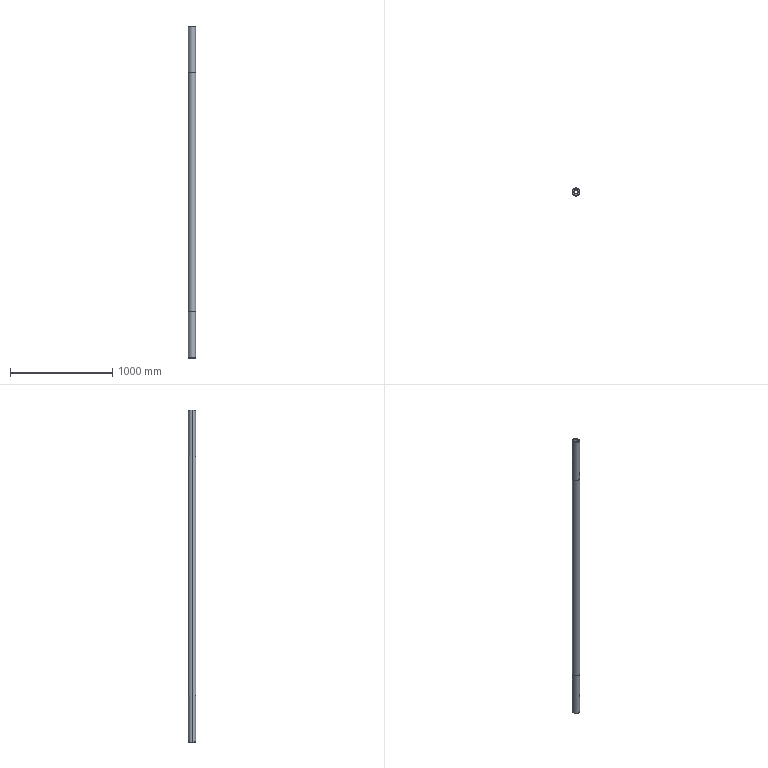Part | SolidWorks | features ICE 4, Chamfer 1, Extrusion 1, MirrorPattern 1 | 1 solid | 31 faces | box 76 x 76 x 3254 mm | volume 9186172 mm3 | cylinder 11 | cone 10 | plane 10 | commonest cylinder face diameters 70 x4 12 x3 44 x2 76 x2
STEP:
#1=CARTESIAN_POINT('',(-34.,0.,0.));
#2=VERTEX_POINT('',#1);
#3=CARTESIAN_POINT('',(-6.,33.466,0.));
#4=VERTEX_POINT('',#3);
#5=CARTESIAN_POINT('',(0.,0.,0.));
#6=DIRECTION('',(0.,0.,-1.));
#7=DIRECTION('',(1.,0.,0.));
#8=AXIS2_PLACEMENT_3D('',#5,#6,#7);
#9=CIRCLE('',#8,34.);
#10=EDGE_CURVE('',#2,#4,#9,.T.);
#11=ORIENTED_EDGE('',*,*,#10,.F.);
#12=CARTESIAN_POINT('',(-35.,0.,1.));
#13=VERTEX_POINT('',#12);
#14=CARTESIAN_POINT('',(-34.,0.,0.));
#15=DIRECTION('',(-0.7071,0.,0.7071));
#16=VECTOR('',#15,1000.);
#17=LINE('',#14,#16);
#18=EDGE_CURVE('',#2,#13,#17,.T.);
#19=ORIENTED_EDGE('',*,*,#18,.T.);
#20=CARTESIAN_POINT('',(-6.,34.482,1.));
#21=VERTEX_POINT('',#20);
#22=CARTESIAN_POINT('',(0.,0.,1.));
#23=DIRECTION('',(0.,0.,1.));
#24=DIRECTION('',(1.,0.,0.));
#25=AXIS2_PLACEMENT_3D('',#22,#23,#24);
#26=CIRCLE('',#25,35.);
#27=EDGE_CURVE('',#21,#13,#26,.T.);
#28=ORIENTED_EDGE('',*,*,#27,.F.);
#29=CARTESIAN_POINT('',(-6.,33.466,0.));
#30=CARTESIAN_POINT('',(-6.,33.805,0.3333));
#31=CARTESIAN_POINT('',(-6.,34.143,0.6666));
#32=CARTESIAN_POINT('',(-6.,34.482,1.));
#33=B_SPLINE_CURVE_WITH_KNOTS('',3,(#29,#30,#31,#32),.UNSPECIFIED.,.F.,.F.,(4,4),(0.,0.001425),.UNSPECIFIED.);
#34=EDGE_CURVE('',#4,#21,#33,.T.);
#35=ORIENTED_EDGE('',*,*,#34,.F.);
#36=EDGE_LOOP('',(#11,#19,#28,#35));
#37=FACE_OUTER_BOUND('',#36,.T.);
#38=CARTESIAN_POINT('',(0.,0.,0.));
#39=DIRECTION('',(0.,0.,1.));
#40=DIRECTION('',(1.,0.,0.));
#41=AXIS2_PLACEMENT_3D('',#38,#39,#40);
#42=CONICAL_SURFACE('',#41,34.,0.7854);
#43=ADVANCED_FACE('',(#37),#42,.T.);
#44=ORIENTED_EDGE('',*,*,#18,.F.);
#45=CARTESIAN_POINT('',(34.,0.,0.));
#46=VERTEX_POINT('',#45);
#47=CARTESIAN_POINT('',(0.,0.,0.));
#48=DIRECTION('',(0.,0.,-1.));
#49=DIRECTION('',(1.,0.,0.));
#50=AXIS2_PLACEMENT_3D('',#47,#48,#49);
#51=CIRCLE('',#50,34.);
#52=EDGE_CURVE('',#46,#2,#51,.T.);
#53=ORIENTED_EDGE('',*,*,#52,.F.);
#54=CARTESIAN_POINT('',(35.,0.,1.));
#55=VERTEX_POINT('',#54);
#56=CARTESIAN_POINT('',(34.,0.,0.));
#57=DIRECTION('',(0.7071,0.,0.7071));
#58=VECTOR('',#57,1000.);
#59=LINE('',#56,#58);
#60=EDGE_CURVE('',#46,#55,#59,.T.);
#61=ORIENTED_EDGE('',*,*,#60,.T.);
#62=CARTESIAN_POINT('',(0.,0.,1.));
#63=DIRECTION('',(0.,0.,1.));
#64=DIRECTION('',(1.,0.,0.));
#65=AXIS2_PLACEMENT_3D('',#62,#63,#64);
#66=CIRCLE('',#65,35.);
#67=EDGE_CURVE('',#13,#55,#66,.T.);
#68=ORIENTED_EDGE('',*,*,#67,.F.);
#69=EDGE_LOOP('',(#44,#53,#61,#68));
#70=FACE_OUTER_BOUND('',#69,.T.);
#71=CARTESIAN_POINT('',(0.,0.,0.));
#72=DIRECTION('',(0.,0.,1.));
#73=DIRECTION('',(1.,0.,0.));
#74=AXIS2_PLACEMENT_3D('',#71,#72,#73);
#75=CONICAL_SURFACE('',#74,34.,0.7854);
#76=ADVANCED_FACE('',(#70),#75,.T.);
#77=CARTESIAN_POINT('',(-37.,0.,453.5));
#78=VERTEX_POINT('',#77);
#79=CARTESIAN_POINT('',(37.,0.,453.5));
#80=VERTEX_POINT('',#79);
#81=CARTESIAN_POINT('',(0.,0.,453.5));
#82=DIRECTION('',(0.,0.,-1.));
#83=DIRECTION('',(-1.,0.,0.));
#84=AXIS2_PLACEMENT_3D('',#81,#82,#83);
#85=CIRCLE('',#84,37.);
#86=EDGE_CURVE('',#78,#80,#85,.T.);
#87=ORIENTED_EDGE('',*,*,#86,.F.);
#88=CARTESIAN_POINT('',(-38.,0.,454.5));
#89=VERTEX_POINT('',#88);
#90=CARTESIAN_POINT('',(-37.,0.,453.5));
#91=DIRECTION('',(-0.7071,0.,0.7071));
#92=VECTOR('',#91,1000.);
#93=LINE('',#90,#92);
#94=EDGE_CURVE('',#78,#89,#93,.T.);
#95=ORIENTED_EDGE('',*,*,#94,.T.);
#96=CARTESIAN_POINT('',(38.,0.,454.5));
#97=VERTEX_POINT('',#96);
#98=CARTESIAN_POINT('',(0.,0.,454.5));
#99=DIRECTION('',(0.,0.,1.));
#100=DIRECTION('',(-1.,0.,0.));
#101=AXIS2_PLACEMENT_3D('',#98,#99,#100);
#102=CIRCLE('',#101,38.);
#103=EDGE_CURVE('',#97,#89,#102,.T.);
#104=ORIENTED_EDGE('',*,*,#103,.F.);
#105=CARTESIAN_POINT('',(37.,0.,453.5));
#106=DIRECTION('',(0.7071,0.,0.7071));
#107=VECTOR('',#106,1000.);
#108=LINE('',#105,#107);
#109=EDGE_CURVE('',#80,#97,#108,.T.);
#110=ORIENTED_EDGE('',*,*,#109,.F.);
#111=EDGE_LOOP('',(#87,#95,#104,#110));
#112=FACE_OUTER_BOUND('',#111,.T.);
#113=CARTESIAN_POINT('',(0.,0.,453.5));
#114=DIRECTION('',(0.,0.,1.));
#115=DIRECTION('',(1.,0.,0.));
#116=AXIS2_PLACEMENT_3D('',#113,#114,#115);
#117=CONICAL_SURFACE('',#116,37.,0.7854);
#118=ADVANCED_FACE('',(#112),#117,.T.);
#119=CARTESIAN_POINT('',(37.,0.,2800.5));
#120=VERTEX_POINT('',#119);
#121=CARTESIAN_POINT('',(-37.,0.,2800.5));
#122=VERTEX_POINT('',#121);
#123=CARTESIAN_POINT('',(0.,0.,2800.5));
#124=DIRECTION('',(0.,0.,1.));
#125=DIRECTION('',(1.,0.,0.));
#126=AXIS2_PLACEMENT_3D('',#123,#124,#125);
#127=CIRCLE('',#126,37.);
#128=EDGE_CURVE('',#120,#122,#127,.T.);
#129=ORIENTED_EDGE('',*,*,#128,.F.);
#130=CARTESIAN_POINT('',(38.,0.,2799.5));
#131=VERTEX_POINT('',#130);
#132=CARTESIAN_POINT('',(37.,0.,2800.5));
#133=DIRECTION('',(0.7071,0.,-0.7071));
#134=VECTOR('',#133,1000.);
#135=LINE('',#132,#134);
#136=EDGE_CURVE('',#120,#131,#135,.T.);
#137=ORIENTED_EDGE('',*,*,#136,.T.);
#138=CARTESIAN_POINT('',(-38.,0.,2799.5));
#139=VERTEX_POINT('',#138);
#140=CARTESIAN_POINT('',(0.,0.,2799.5));
#141=DIRECTION('',(0.,0.,-1.));
#142=DIRECTION('',(1.,0.,0.));
#143=AXIS2_PLACEMENT_3D('',#140,#141,#142);
#144=CIRCLE('',#143,38.);
#145=EDGE_CURVE('',#139,#131,#144,.T.);
#146=ORIENTED_EDGE('',*,*,#145,.F.);
#147=CARTESIAN_POINT('',(-37.,0.,2800.5));
#148=DIRECTION('',(-0.7071,0.,-0.7071));
#149=VECTOR('',#148,1000.);
#150=LINE('',#147,#149);
#151=EDGE_CURVE('',#122,#139,#150,.T.);
#152=ORIENTED_EDGE('',*,*,#151,.F.);
#153=EDGE_LOOP('',(#129,#137,#146,#152));
#154=FACE_OUTER_BOUND('',#153,.T.);
#155=CARTESIAN_POINT('',(0.,0.,2800.5));
#156=DIRECTION('',(0.,0.,-1.));
#157=DIRECTION('',(-1.,0.,0.));
#158=AXIS2_PLACEMENT_3D('',#155,#156,#157);
#159=CONICAL_SURFACE('',#158,37.,0.7854);
#160=ADVANCED_FACE('',(#154),#159,.T.);
#161=CARTESIAN_POINT('',(34.,0.,3254.));
#162=VERTEX_POINT('',#161);
#163=CARTESIAN_POINT('',(6.,33.466,3254.));
#164=VERTEX_POINT('',#163);
#165=CARTESIAN_POINT('',(0.,0.,3254.));
#166=DIRECTION('',(0.,0.,1.));
#167=DIRECTION('',(1.,0.,0.));
#168=AXIS2_PLACEMENT_3D('',#165,#166,#167);
#169=CIRCLE('',#168,34.);
#170=EDGE_CURVE('',#162,#164,#169,.T.);
#171=ORIENTED_EDGE('',*,*,#170,.F.);
#172=CARTESIAN_POINT('',(35.,0.,3253.));
#173=VERTEX_POINT('',#172);
#174=CARTESIAN_POINT('',(34.,0.,3254.));
#175=DIRECTION('',(0.7071,0.,-0.7071));
#176=VECTOR('',#175,1000.);
#177=LINE('',#174,#176);
#178=EDGE_CURVE('',#162,#173,#177,.T.);
#179=ORIENTED_EDGE('',*,*,#178,.T.);
#180=CARTESIAN_POINT('',(6.,34.482,3253.));
#181=VERTEX_POINT('',#180);
#182=CARTESIAN_POINT('',(0.,0.,3253.));
#183=DIRECTION('',(0.,0.,-1.));
#184=DIRECTION('',(1.,0.,0.));
#185=AXIS2_PLACEMENT_3D('',#182,#183,#184);
#186=CIRCLE('',#185,35.);
#187=EDGE_CURVE('',#181,#173,#186,.T.);
#188=ORIENTED_EDGE('',*,*,#187,.F.);
#189=CARTESIAN_POINT('',(6.,33.466,3254.));
#190=CARTESIAN_POINT('',(6.,33.805,3253.667));
#191=CARTESIAN_POINT('',(6.,34.143,3253.333));
#192=CARTESIAN_POINT('',(6.,34.482,3253.));
#193=B_SPLINE_CURVE_WITH_KNOTS('',3,(#189,#190,#191,#192),.UNSPECIFIED.,.F.,.F.,(4,4),(0.,0.001425),.UNSPECIFIED.);
#194=EDGE_CURVE('',#164,#181,#193,.T.);
#195=ORIENTED_EDGE('',*,*,#194,.F.);
#196=EDGE_LOOP('',(#171,#179,#188,#195));
#197=FACE_OUTER_BOUND('',#196,.T.);
#198=CARTESIAN_POINT('',(0.,0.,3254.));
#199=DIRECTION('',(0.,0.,-1.));
#200=DIRECTION('',(-1.,0.,0.));
#201=AXIS2_PLACEMENT_3D('',#198,#199,#200);
#202=CONICAL_SURFACE('',#201,34.,0.7854);
#203=ADVANCED_FACE('',(#197),#202,.T.);
#204=ORIENTED_EDGE('',*,*,#178,.F.);
#205=CARTESIAN_POINT('',(-34.,0.,3254.));
#206=VERTEX_POINT('',#205);
#207=CARTESIAN_POINT('',(0.,0.,3254.));
#208=DIRECTION('',(0.,0.,1.));
#209=DIRECTION('',(1.,0.,0.));
#210=AXIS2_PLACEMENT_3D('',#207,#208,#209);
#211=CIRCLE('',#210,34.);
#212=EDGE_CURVE('',#206,#162,#211,.T.);
#213=ORIENTED_EDGE('',*,*,#212,.F.);
#214=CARTESIAN_POINT('',(-35.,0.,3253.));
#215=VERTEX_POINT('',#214);
#216=CARTESIAN_POINT('',(-34.,0.,3254.));
#217=DIRECTION('',(-0.7071,0.,-0.7071));
#218=VECTOR('',#217,1000.);
#219=LINE('',#216,#218);
#220=EDGE_CURVE('',#206,#215,#219,.T.);
#221=ORIENTED_EDGE('',*,*,#220,.T.);
#222=CARTESIAN_POINT('',(0.,0.,3253.));
#223=DIRECTION('',(0.,0.,-1.));
#224=DIRECTION('',(1.,0.,0.));
#225=AXIS2_PLACEMENT_3D('',#222,#223,#224);
#226=CIRCLE('',#225,35.);
#227=EDGE_CURVE('',#173,#215,#226,.T.);
#228=ORIENTED_EDGE('',*,*,#227,.F.);
#229=EDGE_LOOP('',(#204,#213,#221,#228));
#230=FACE_OUTER_BOUND('',#229,.T.);
#231=CARTESIAN_POINT('',(0.,0.,3254.));
#232=DIRECTION('',(0.,0.,-1.));
#233=DIRECTION('',(-1.,0.,0.));
#234=AXIS2_PLACEMENT_3D('',#231,#232,#233);
#235=CONICAL_SURFACE('',#234,34.,0.7854);
#236=ADVANCED_FACE('',(#230),#235,.T.);
#237=CARTESIAN_POINT('',(0.,31.,36.));
#238=VERTEX_POINT('',#237);
#239=CARTESIAN_POINT('',(6.,31.,30.));
#240=VERTEX_POINT('',#239);
#241=CARTESIAN_POINT('',(0.,31.,30.));
#242=DIRECTION('',(0.,1.,0.));
#243=DIRECTION('',(0.,0.,1.));
#244=AXIS2_PLACEMENT_3D('',#241,#242,#243);
#245=CIRCLE('',#244,6.);
#246=EDGE_CURVE('',#238,#240,#245,.T.);
#247=ORIENTED_EDGE('',*,*,#246,.F.);
#248=CARTESIAN_POINT('',(0.,35.,36.));
#249=VERTEX_POINT('',#248);
#250=CARTESIAN_POINT('',(0.,31.,36.));
#251=DIRECTION('',(0.,1.,0.));
#252=VECTOR('',#251,1000.);
#253=LINE('',#250,#252);
#254=EDGE_CURVE('',#238,#249,#253,.T.);
#255=ORIENTED_EDGE('',*,*,#254,.T.);
#256=CARTESIAN_POINT('',(6.,34.482,30.));
#257=VERTEX_POINT('',#256);
#258=CARTESIAN_POINT('',(0.,35.,36.));
#259=CARTESIAN_POINT('',(0.3919,35.,36.));
#260=CARTESIAN_POINT('',(0.79,34.993,35.961));
#261=CARTESIAN_POINT('',(1.559,34.967,35.807));
#262=CARTESIAN_POINT('',(1.934,34.948,35.694));
#263=CARTESIAN_POINT('',(2.479,34.913,35.468));
#264=CARTESIAN_POINT('',(2.658,34.899,35.383));
#265=CARTESIAN_POINT('',(3.005,34.871,35.197));
#266=CARTESIAN_POINT('',(3.173,34.856,35.096));
#267=CARTESIAN_POINT('',(3.659,34.81,34.771));
#268=CARTESIAN_POINT('',(3.963,34.776,34.522));
#269=CARTESIAN_POINT('',(4.521,34.708,33.964));
#270=CARTESIAN_POINT('',(4.769,34.674,33.662));
#271=CARTESIAN_POINT('',(5.094,34.627,33.176));
#272=CARTESIAN_POINT('',(5.195,34.612,33.008));
#273=CARTESIAN_POINT('',(5.381,34.584,32.661));
#274=CARTESIAN_POINT('',(5.466,34.571,32.482));
#275=CARTESIAN_POINT('',(5.692,34.534,31.938));
#276=CARTESIAN_POINT('',(5.806,34.515,31.564));
#277=CARTESIAN_POINT('',(5.96,34.489,30.794));
#278=CARTESIAN_POINT('',(6.,34.482,30.397));
#279=CARTESIAN_POINT('',(6.,34.482,30.));
#280=B_SPLINE_CURVE_WITH_KNOTS('',3,(#258,#259,#260,#261,#262,#263,#264,#265,#266,#267,#268,#269,#270,#271,#272,#273,#274,#275,#276,#277,#278,#279),.UNSPECIFIED.,.F.,.F.,(4,2,2,2,2,2,2,2,2,2,4),(0.009399,0.01057,0.01175,0.01233,0.01292,0.01409,0.01527,0.01585,0.01644,0.01761,0.01879),.UNSPECIFIED.);
#281=EDGE_CURVE('',#249,#257,#280,.T.);
#282=ORIENTED_EDGE('',*,*,#281,.T.);
#283=CARTESIAN_POINT('',(6.,31.,30.));
#284=DIRECTION('',(0.,1.,0.));
#285=VECTOR('',#284,1000.);
#286=LINE('',#283,#285);
#287=EDGE_CURVE('',#240,#257,#286,.T.);
#288=ORIENTED_EDGE('',*,*,#287,.F.);
#289=EDGE_LOOP('',(#247,#255,#282,#288));
#290=FACE_OUTER_BOUND('',#289,.T.);
#291=CARTESIAN_POINT('',(0.,31.,30.));
#292=DIRECTION('',(0.,1.,0.));
#293=DIRECTION('',(0.,0.,1.));
#294=AXIS2_PLACEMENT_3D('',#291,#292,#293);
#295=CYLINDRICAL_SURFACE('',#294,6.);
#296=ADVANCED_FACE('',(#290),#295,.F.);
#297=CARTESIAN_POINT('',(22.,0.,3254.));
#298=VERTEX_POINT('',#297);
#299=CARTESIAN_POINT('',(-22.,0.,3254.));
#300=VERTEX_POINT('',#299);
#301=CARTESIAN_POINT('',(0.,0.,3254.));
#302=DIRECTION('',(0.,0.,-1.));
#303=DIRECTION('',(-1.,0.,0.));
#304=AXIS2_PLACEMENT_3D('',#301,#302,#303);
#305=CIRCLE('',#304,22.);
#306=EDGE_CURVE('',#298,#300,#305,.T.);
#307=ORIENTED_EDGE('',*,*,#306,.F.);
#308=CARTESIAN_POINT('',(22.,0.,0.));
#309=VERTEX_POINT('',#308);
#310=CARTESIAN_POINT('',(22.,0.,3254.));
#311=DIRECTION('',(0.,0.,-1.));
#312=VECTOR('',#311,1000.);
#313=LINE('',#310,#312);
#314=EDGE_CURVE('',#298,#309,#313,.T.);
#315=ORIENTED_EDGE('',*,*,#314,.T.);
#316=CARTESIAN_POINT('',(-22.,0.,0.));
#317=VERTEX_POINT('',#316);
#318=CARTESIAN_POINT('',(0.,0.,0.));
#319=DIRECTION('',(0.,0.,-1.));
#320=DIRECTION('',(-1.,0.,0.));
#321=AXIS2_PLACEMENT_3D('',#318,#319,#320);
#322=CIRCLE('',#321,22.);
#323=EDGE_CURVE('',#309,#317,#322,.T.);
#324=ORIENTED_EDGE('',*,*,#323,.T.);
#325=CARTESIAN_POINT('',(-22.,0.,3254.));
#326=DIRECTION('',(0.,0.,-1.));
#327=VECTOR('',#326,1000.);
#328=LINE('',#325,#327);
#329=EDGE_CURVE('',#300,#317,#328,.T.);
#330=ORIENTED_EDGE('',*,*,#329,.F.);
#331=EDGE_LOOP('',(#307,#315,#324,#330));
#332=FACE_OUTER_BOUND('',#331,.T.);
#333=CARTESIAN_POINT('',(0.,0.,3254.));
#334=DIRECTION('',(0.,0.,-1.));
#335=DIRECTION('',(-1.,0.,0.));
#336=AXIS2_PLACEMENT_3D('',#333,#334,#335);
#337=CYLINDRICAL_SURFACE('',#336,22.);
#338=ADVANCED_FACE('',(#332),#337,.F.);
#339=CARTESIAN_POINT('',(-35.,0.,453.5));
#340=VERTEX_POINT('',#339);
#341=CARTESIAN_POINT('',(35.,0.,453.5));
#342=VERTEX_POINT('',#341);
#343=CARTESIAN_POINT('',(0.,0.,453.5));
#344=DIRECTION('',(0.,0.,-1.));
#345=DIRECTION('',(-1.,0.,0.));
#346=AXIS2_PLACEMENT_3D('',#343,#344,#345);
#347=CIRCLE('',#346,35.);
#348=EDGE_CURVE('',#340,#342,#347,.T.);
#349=ORIENTED_EDGE('',*,*,#348,.T.);
#350=CARTESIAN_POINT('',(35.,0.,453.5));
#351=DIRECTION('',(0.,0.,-1.));
#352=VECTOR('',#351,1000.);
#353=LINE('',#350,#352);
#354=EDGE_CURVE('',#342,#55,#353,.T.);
#355=ORIENTED_EDGE('',*,*,#354,.T.);
#356=CARTESIAN_POINT('',(6.,34.482,1.));
#357=VERTEX_POINT('',#356);
#358=CARTESIAN_POINT('',(0.,0.,1.));
#359=DIRECTION('',(0.,0.,1.));
#360=DIRECTION('',(1.,0.,0.));
#361=AXIS2_PLACEMENT_3D('',#358,#359,#360);
#362=CIRCLE('',#361,35.);
#363=EDGE_CURVE('',#55,#357,#362,.T.);
#364=ORIENTED_EDGE('',*,*,#363,.T.);
#365=CARTESIAN_POINT('',(6.,34.482,453.5));
#366=DIRECTION('',(0.,0.,-1.));
#367=VECTOR('',#366,1000.);
#368=LINE('',#365,#367);
#369=EDGE_CURVE('',#257,#357,#368,.T.);
#370=ORIENTED_EDGE('',*,*,#369,.F.);
#371=ORIENTED_EDGE('',*,*,#281,.F.);
#372=CARTESIAN_POINT('',(-6.,34.482,30.));
#373=VERTEX_POINT('',#372);
#374=CARTESIAN_POINT('',(-6.,34.482,30.));
#375=CARTESIAN_POINT('',(-6.,34.482,30.397));
#376=CARTESIAN_POINT('',(-5.961,34.489,30.788));
#377=CARTESIAN_POINT('',(-5.846,34.508,31.364));
#378=CARTESIAN_POINT('',(-5.799,34.516,31.554));
#379=CARTESIAN_POINT('',(-5.684,34.535,31.932));
#380=CARTESIAN_POINT('',(-5.617,34.546,32.119));
#381=CARTESIAN_POINT('',(-5.391,34.583,32.664));
#382=CARTESIAN_POINT('',(-5.206,34.611,33.008));
#383=CARTESIAN_POINT('',(-4.77,34.674,33.66));
#384=CARTESIAN_POINT('',(-4.517,34.708,33.968));
#385=CARTESIAN_POINT('',(-3.965,34.776,34.521));
#386=CARTESIAN_POINT('',(-3.663,34.809,34.769));
#387=CARTESIAN_POINT('',(-3.007,34.872,35.207));
#388=CARTESIAN_POINT('',(-2.659,34.901,35.393));
#389=CARTESIAN_POINT('',(-2.117,34.936,35.618));
#390=CARTESIAN_POINT('',(-1.933,34.947,35.684));
#391=CARTESIAN_POINT('',(-1.557,34.966,35.798));
#392=CARTESIAN_POINT('',(-1.364,34.974,35.846));
#393=CARTESIAN_POINT('',(-0.7822,34.993,35.962));
#394=CARTESIAN_POINT('',(-0.3923,35.,36.));
#395=CARTESIAN_POINT('',(0.,35.,36.));
#396=B_SPLINE_CURVE_WITH_KNOTS('',3,(#374,#375,#376,#377,#378,#379,#380,#381,#382,#383,#384,#385,#386,#387,#388,#389,#390,#391,#392,#393,#394,#395),.UNSPECIFIED.,.F.,.F.,(4,2,2,2,2,2,2,2,2,2,4),(0.,0.001175,0.001762,0.00235,0.003525,0.004699,0.005874,0.007049,0.007637,0.008224,0.009399),.UNSPECIFIED.);
#397=EDGE_CURVE('',#373,#249,#396,.T.);
#398=ORIENTED_EDGE('',*,*,#397,.F.);
#399=CARTESIAN_POINT('',(-6.,34.482,453.5));
#400=DIRECTION('',(0.,0.,1.));
#401=VECTOR('',#400,1000.);
#402=LINE('',#399,#401);
#403=EDGE_CURVE('',#21,#373,#402,.T.);
#404=ORIENTED_EDGE('',*,*,#403,.F.);
#405=ORIENTED_EDGE('',*,*,#27,.T.);
#406=CARTESIAN_POINT('',(-35.,0.,453.5));
#407=DIRECTION('',(0.,0.,-1.));
#408=VECTOR('',#407,1000.);
#409=LINE('',#406,#408);
#410=EDGE_CURVE('',#340,#13,#409,.T.);
#411=ORIENTED_EDGE('',*,*,#410,.F.);
#412=EDGE_LOOP('',(#349,#355,#364,#370,#371,#398,#404,#405,#411));
#413=FACE_OUTER_BOUND('',#412,.T.);
#414=CARTESIAN_POINT('',(0.,0.,453.5));
#415=DIRECTION('',(0.,0.,-1.));
#416=DIRECTION('',(-1.,0.,0.));
#417=AXIS2_PLACEMENT_3D('',#414,#415,#416);
#418=CYLINDRICAL_SURFACE('',#417,35.);
#419=ADVANCED_FACE('',(#413),#418,.T.);
#420=ORIENTED_EDGE('',*,*,#145,.T.);
#421=CARTESIAN_POINT('',(38.,0.,3254.));
#422=DIRECTION('',(0.,0.,-1.));
#423=VECTOR('',#422,1000.);
#424=LINE('',#421,#423);
#425=EDGE_CURVE('',#131,#97,#424,.T.);
#426=ORIENTED_EDGE('',*,*,#425,.T.);
#427=ORIENTED_EDGE('',*,*,#103,.T.);
#428=CARTESIAN_POINT('',(-38.,0.,3254.));
#429=DIRECTION('',(0.,0.,-1.));
#430=VECTOR('',#429,1000.);
#431=LINE('',#428,#430);
#432=EDGE_CURVE('',#139,#89,#431,.T.);
#433=ORIENTED_EDGE('',*,*,#432,.F.);
#434=EDGE_LOOP('',(#420,#426,#427,#433));
#435=FACE_OUTER_BOUND('',#434,.T.);
#436=CARTESIAN_POINT('',(0.,0.,3254.));
#437=DIRECTION('',(0.,0.,-1.));
#438=DIRECTION('',(-1.,0.,0.));
#439=AXIS2_PLACEMENT_3D('',#436,#437,#438);
#440=CYLINDRICAL_SURFACE('',#439,38.);
#441=ADVANCED_FACE('',(#435),#440,.T.);
#442=CARTESIAN_POINT('',(35.,0.,2800.5));
#443=VERTEX_POINT('',#442);
#444=CARTESIAN_POINT('',(-35.,0.,2800.5));
#445=VERTEX_POINT('',#444);
#446=CARTESIAN_POINT('',(0.,0.,2800.5));
#447=DIRECTION('',(0.,0.,1.));
#448=DIRECTION('',(1.,0.,0.));
#449=AXIS2_PLACEMENT_3D('',#446,#447,#448);
#450=CIRCLE('',#449,35.);
#451=EDGE_CURVE('',#443,#445,#450,.T.);
#452=ORIENTED_EDGE('',*,*,#451,.T.);
#453=CARTESIAN_POINT('',(-35.,0.,2800.5));
#454=DIRECTION('',(0.,0.,1.));
#455=VECTOR('',#454,1000.);
#456=LINE('',#453,#455);
#457=EDGE_CURVE('',#445,#215,#456,.T.);
#458=ORIENTED_EDGE('',*,*,#457,.T.);
#459=CARTESIAN_POINT('',(-6.,34.482,3253.));
#460=VERTEX_POINT('',#459);
#461=CARTESIAN_POINT('',(0.,0.,3253.));
#462=DIRECTION('',(0.,0.,-1.));
#463=DIRECTION('',(1.,0.,0.));
#464=AXIS2_PLACEMENT_3D('',#461,#462,#463);
#465=CIRCLE('',#464,35.);
#466=EDGE_CURVE('',#215,#460,#465,.T.);
#467=ORIENTED_EDGE('',*,*,#466,.T.);
#468=CARTESIAN_POINT('',(-6.,34.482,3224.));
#469=VERTEX_POINT('',#468);
#470=CARTESIAN_POINT('',(-6.,34.482,2800.5));
#471=DIRECTION('',(0.,0.,-1.));
#472=VECTOR('',#471,1000.);
#473=LINE('',#470,#472);
#474=EDGE_CURVE('',#460,#469,#473,.T.);
#475=ORIENTED_EDGE('',*,*,#474,.T.);
#476=CARTESIAN_POINT('',(6.,34.482,3224.));
#477=VERTEX_POINT('',#476);
#478=CARTESIAN_POINT('',(-6.,34.482,3224.));
#479=CARTESIAN_POINT('',(-6.,34.482,3223.603));
#480=CARTESIAN_POINT('',(-5.961,34.489,3223.213));
#481=CARTESIAN_POINT('',(-5.846,34.508,3222.637));
#482=CARTESIAN_POINT('',(-5.799,34.516,3222.446));
#483=CARTESIAN_POINT('',(-5.684,34.535,3222.069));
#484=CARTESIAN_POINT('',(-5.617,34.546,3221.882));
#485=CARTESIAN_POINT('',(-5.391,34.583,3221.337));
#486=CARTESIAN_POINT('',(-5.207,34.611,3220.993));
#487=CARTESIAN_POINT('',(-4.772,34.674,3220.341));
#488=CARTESIAN_POINT('',(-4.519,34.708,3220.033));
#489=CARTESIAN_POINT('',(-3.966,34.776,3219.481));
#490=CARTESIAN_POINT('',(-3.665,34.809,3219.233));
#491=CARTESIAN_POINT('',(-3.009,34.872,3218.794));
#492=CARTESIAN_POINT('',(-2.661,34.901,3218.608));
#493=CARTESIAN_POINT('',(-2.12,34.936,3218.384));
#494=CARTESIAN_POINT('',(-1.936,34.947,3218.318));
#495=CARTESIAN_POINT('',(-1.56,34.966,3218.203));
#496=CARTESIAN_POINT('',(-1.367,34.974,3218.155));
#497=CARTESIAN_POINT('',(-0.7864,34.993,3218.039));
#498=CARTESIAN_POINT('',(-0.3967,35.,3218.));
#499=CARTESIAN_POINT('',(0.3874,35.,3218.));
#500=CARTESIAN_POINT('',(0.7857,34.993,3218.039));
#501=CARTESIAN_POINT('',(1.556,34.968,3218.192));
#502=CARTESIAN_POINT('',(1.93,34.949,3218.305));
#503=CARTESIAN_POINT('',(2.476,34.913,3218.531));
#504=CARTESIAN_POINT('',(2.655,34.9,3218.616));
#505=CARTESIAN_POINT('',(3.002,34.871,3218.801));
#506=CARTESIAN_POINT('',(3.17,34.857,3218.902));
#507=CARTESIAN_POINT('',(3.657,34.81,3219.227));
#508=CARTESIAN_POINT('',(3.961,34.776,3219.476));
#509=CARTESIAN_POINT('',(4.52,34.708,3220.034));
#510=CARTESIAN_POINT('',(4.767,34.674,3220.336));
#511=CARTESIAN_POINT('',(5.093,34.628,3220.823));
#512=CARTESIAN_POINT('',(5.194,34.613,3220.99));
#513=CARTESIAN_POINT('',(5.381,34.584,3221.338));
#514=CARTESIAN_POINT('',(5.466,34.571,3221.517));
#515=CARTESIAN_POINT('',(5.692,34.534,3222.061));
#516=CARTESIAN_POINT('',(5.806,34.515,3222.435));
#517=CARTESIAN_POINT('',(5.96,34.489,3223.205));
#518=CARTESIAN_POINT('',(6.,34.482,3223.603));
#519=CARTESIAN_POINT('',(6.,34.482,3224.));
#520=B_SPLINE_CURVE_WITH_KNOTS('',3,(#478,#479,#480,#481,#482,#483,#484,#485,#486,#487,#488,#489,#490,#491,#492,#493,#494,#495,#496,#497,#498,#499,#500,#501,#502,#503,#504,#505,#506,#507,#508,#509,#510,#511,#512,#513,#514,#515,#516,#517,#518,#519),.UNSPECIFIED.,.F.,.F.,(4,2,2,2,2,2,2,2,2,2,2,2,2,2,2,2,2,2,2,2,4),(0.,0.001174,0.001761,0.002349,0.003523,0.004697,0.005871,0.007046,0.007633,0.00822,0.009394,0.01057,0.01174,0.01233,0.01292,0.01409,0.01527,0.01585,0.01644,0.01761,0.01879),.UNSPECIFIED.);
#521=EDGE_CURVE('',#469,#477,#520,.T.);
#522=ORIENTED_EDGE('',*,*,#521,.T.);
#523=CARTESIAN_POINT('',(6.,34.482,2800.5));
#524=DIRECTION('',(0.,0.,1.));
#525=VECTOR('',#524,1000.);
#526=LINE('',#523,#525);
#527=EDGE_CURVE('',#477,#181,#526,.T.);
#528=ORIENTED_EDGE('',*,*,#527,.T.);
#529=ORIENTED_EDGE('',*,*,#187,.T.);
#530=CARTESIAN_POINT('',(35.,0.,2800.5));
#531=DIRECTION('',(0.,0.,1.));
#532=VECTOR('',#531,1000.);
#533=LINE('',#530,#532);
#534=EDGE_CURVE('',#443,#173,#533,.T.);
#535=ORIENTED_EDGE('',*,*,#534,.F.);
#536=EDGE_LOOP('',(#452,#458,#467,#475,#522,#528,#529,#535));
#537=FACE_OUTER_BOUND('',#536,.T.);
#538=CARTESIAN_POINT('',(0.,0.,2800.5));
#539=DIRECTION('',(0.,0.,1.));
#540=DIRECTION('',(1.,0.,0.));
#541=AXIS2_PLACEMENT_3D('',#538,#539,#540);
#542=CYLINDRICAL_SURFACE('',#541,35.);
#543=ADVANCED_FACE('',(#537),#542,.T.);
#544=ORIENTED_EDGE('',*,*,#457,.F.);
#545=CARTESIAN_POINT('',(0.,0.,2800.5));
#546=DIRECTION('',(0.,0.,1.));
#547=DIRECTION('',(1.,0.,0.));
#548=AXIS2_PLACEMENT_3D('',#545,#546,#547);
#549=CIRCLE('',#548,35.);
#550=EDGE_CURVE('',#445,#443,#549,.T.);
#551=ORIENTED_EDGE('',*,*,#550,.T.);
#552=ORIENTED_EDGE('',*,*,#534,.T.);
#553=ORIENTED_EDGE('',*,*,#227,.T.);
#554=EDGE_LOOP('',(#544,#551,#552,#553));
#555=FACE_OUTER_BOUND('',#554,.T.);
#556=CARTESIAN_POINT('',(0.,0.,2800.5));
#557=DIRECTION('',(0.,0.,1.));
#558=DIRECTION('',(1.,0.,0.));
#559=AXIS2_PLACEMENT_3D('',#556,#557,#558);
#560=CYLINDRICAL_SURFACE('',#559,35.);
#561=ADVANCED_FACE('',(#555),#560,.T.);
#562=CARTESIAN_POINT('',(0.,0.,3254.));
#563=DIRECTION('',(0.,0.,-1.));
#564=DIRECTION('',(-1.,0.,0.));
#565=AXIS2_PLACEMENT_3D('',#562,#563,#564);
#566=CIRCLE('',#565,22.);
#567=EDGE_CURVE('',#300,#298,#566,.T.);
#568=ORIENTED_EDGE('',*,*,#567,.T.);
#569=ORIENTED_EDGE('',*,*,#306,.T.);
#570=EDGE_LOOP('',(#568,#569));
#571=FACE_BOUND('',#570,.T.);
#572=CARTESIAN_POINT('',(-6.,31.,3254.));
#573=VERTEX_POINT('',#572);
#574=CARTESIAN_POINT('',(-6.,33.466,3254.));
#575=VERTEX_POINT('',#574);
#576=CARTESIAN_POINT('',(-6.,31.,3254.));
#577=DIRECTION('',(0.,1.,0.));
#578=VECTOR('',#577,1000.);
#579=LINE('',#576,#578);
#580=EDGE_CURVE('',#573,#575,#579,.T.);
#581=ORIENTED_EDGE('',*,*,#580,.T.);
#582=CARTESIAN_POINT('',(0.,0.,3254.));
#583=DIRECTION('',(0.,0.,1.));
#584=DIRECTION('',(1.,0.,0.));
#585=AXIS2_PLACEMENT_3D('',#582,#583,#584);
#586=CIRCLE('',#585,34.);
#587=EDGE_CURVE('',#575,#206,#586,.T.);
#588=ORIENTED_EDGE('',*,*,#587,.T.);
#589=ORIENTED_EDGE('',*,*,#212,.T.);
#590=ORIENTED_EDGE('',*,*,#170,.T.);
#591=CARTESIAN_POINT('',(6.,31.,3254.));
#592=VERTEX_POINT('',#591);
#593=CARTESIAN_POINT('',(6.,31.,3254.));
#594=DIRECTION('',(0.,1.,0.));
#595=VECTOR('',#594,1000.);
#596=LINE('',#593,#595);
#597=EDGE_CURVE('',#592,#164,#596,.T.);
#598=ORIENTED_EDGE('',*,*,#597,.F.);
#599=CARTESIAN_POINT('',(0.,31.,3254.));
#600=DIRECTION('',(-1.,0.,0.));
#601=VECTOR('',#600,1000.);
#602=LINE('',#599,#601);
#603=EDGE_CURVE('',#592,#573,#602,.T.);
#604=ORIENTED_EDGE('',*,*,#603,.T.);
#605=EDGE_LOOP('',(#581,#588,#589,#590,#598,#604));
#606=FACE_OUTER_BOUND('',#605,.T.);
#607=CARTESIAN_POINT('',(0.,0.,3254.));
#608=DIRECTION('',(0.,0.,1.));
#609=DIRECTION('',(1.,0.,0.));
#610=AXIS2_PLACEMENT_3D('',#607,#608,#609);
#611=PLANE('',#610);
#612=ADVANCED_FACE('',(#571,#606),#611,.T.);
#613=ORIENTED_EDGE('',*,*,#425,.F.);
#614=CARTESIAN_POINT('',(0.,0.,2799.5));
#615=DIRECTION('',(0.,0.,-1.));
#616=DIRECTION('',(1.,0.,0.));
#617=AXIS2_PLACEMENT_3D('',#614,#615,#616);
#618=CIRCLE('',#617,38.);
#619=EDGE_CURVE('',#131,#139,#618,.T.);
#620=ORIENTED_EDGE('',*,*,#619,.T.);
#621=ORIENTED_EDGE('',*,*,#432,.T.);
#622=CARTESIAN_POINT('',(0.,0.,454.5));
#623=DIRECTION('',(0.,0.,1.));
#624=DIRECTION('',(-1.,0.,0.));
#625=AXIS2_PLACEMENT_3D('',#622,#623,#624);
#626=CIRCLE('',#625,38.);
#627=EDGE_CURVE('',#89,#97,#626,.T.);
#628=ORIENTED_EDGE('',*,*,#627,.T.);
#629=EDGE_LOOP('',(#613,#620,#621,#628));
#630=FACE_OUTER_BOUND('',#629,.T.);
#631=CARTESIAN_POINT('',(0.,0.,3254.));
#632=DIRECTION('',(0.,0.,-1.));
#633=DIRECTION('',(-1.,0.,0.));
#634=AXIS2_PLACEMENT_3D('',#631,#632,#633);
#635=CYLINDRICAL_SURFACE('',#634,38.);
#636=ADVANCED_FACE('',(#630),#635,.T.);
#637=CARTESIAN_POINT('',(0.,0.,453.5));
#638=DIRECTION('',(0.,0.,-1.));
#639=DIRECTION('',(-1.,0.,0.));
#640=AXIS2_PLACEMENT_3D('',#637,#638,#639);
#641=CIRCLE('',#640,37.);
#642=EDGE_CURVE('',#80,#78,#641,.T.);
#643=ORIENTED_EDGE('',*,*,#642,.T.);
#644=ORIENTED_EDGE('',*,*,#86,.T.);
#645=EDGE_LOOP('',(#643,#644));
#646=FACE_OUTER_BOUND('',#645,.T.);
#647=ORIENTED_EDGE('',*,*,#348,.F.);
#648=CARTESIAN_POINT('',(0.,0.,453.5));
#649=DIRECTION('',(0.,0.,-1.));
#650=DIRECTION('',(-1.,0.,0.));
#651=AXIS2_PLACEMENT_3D('',#648,#649,#650);
#652=CIRCLE('',#651,35.);
#653=EDGE_CURVE('',#342,#340,#652,.T.);
#654=ORIENTED_EDGE('',*,*,#653,.F.);
#655=EDGE_LOOP('',(#647,#654));
#656=FACE_BOUND('',#655,.T.);
#657=CARTESIAN_POINT('',(0.,0.,453.5));
#658=DIRECTION('',(0.,0.,-1.));
#659=DIRECTION('',(-1.,0.,0.));
#660=AXIS2_PLACEMENT_3D('',#657,#658,#659);
#661=PLANE('',#660);
#662=ADVANCED_FACE('',(#646,#656),#661,.T.);
#663=ORIENTED_EDGE('',*,*,#354,.F.);
#664=ORIENTED_EDGE('',*,*,#653,.T.);
#665=ORIENTED_EDGE('',*,*,#410,.T.);
#666=ORIENTED_EDGE('',*,*,#67,.T.);
#667=EDGE_LOOP('',(#663,#664,#665,#666));
#668=FACE_OUTER_BOUND('',#667,.T.);
#669=CARTESIAN_POINT('',(0.,0.,453.5));
#670=DIRECTION('',(0.,0.,-1.));
#671=DIRECTION('',(-1.,0.,0.));
#672=AXIS2_PLACEMENT_3D('',#669,#670,#671);
#673=CYLINDRICAL_SURFACE('',#672,35.);
#674=ADVANCED_FACE('',(#668),#673,.T.);
#675=CARTESIAN_POINT('',(0.,0.,0.));
#676=DIRECTION('',(0.,0.,-1.));
#677=DIRECTION('',(-1.,0.,0.));
#678=AXIS2_PLACEMENT_3D('',#675,#676,#677);
#679=CIRCLE('',#678,22.);
#680=EDGE_CURVE('',#317,#309,#679,.T.);
#681=ORIENTED_EDGE('',*,*,#680,.F.);
#682=ORIENTED_EDGE('',*,*,#323,.F.);
#683=EDGE_LOOP('',(#681,#682));
#684=FACE_BOUND('',#683,.T.);
#685=CARTESIAN_POINT('',(6.,31.,0.));
#686=VERTEX_POINT('',#685);
#687=CARTESIAN_POINT('',(6.,33.466,0.));
#688=VERTEX_POINT('',#687);
#689=CARTESIAN_POINT('',(6.,31.,0.));
#690=DIRECTION('',(0.,1.,0.));
#691=VECTOR('',#690,1000.);
#692=LINE('',#689,#691);
#693=EDGE_CURVE('',#686,#688,#692,.T.);
#694=ORIENTED_EDGE('',*,*,#693,.T.);
#695=CARTESIAN_POINT('',(0.,0.,0.));
#696=DIRECTION('',(0.,0.,-1.));
#697=DIRECTION('',(1.,0.,0.));
#698=AXIS2_PLACEMENT_3D('',#695,#696,#697);
#699=CIRCLE('',#698,34.);
#700=EDGE_CURVE('',#688,#46,#699,.T.);
#701=ORIENTED_EDGE('',*,*,#700,.T.);
#702=ORIENTED_EDGE('',*,*,#52,.T.);
#703=ORIENTED_EDGE('',*,*,#10,.T.);
#704=CARTESIAN_POINT('',(-6.,31.,0.));
#705=VERTEX_POINT('',#704);
#706=CARTESIAN_POINT('',(-6.,31.,0.));
#707=DIRECTION('',(0.,1.,0.));
#708=VECTOR('',#707,1000.);
#709=LINE('',#706,#708);
#710=EDGE_CURVE('',#705,#4,#709,.T.);
#711=ORIENTED_EDGE('',*,*,#710,.F.);
#712=CARTESIAN_POINT('',(0.,31.,0.));
#713=DIRECTION('',(-1.,0.,0.));
#714=VECTOR('',#713,1000.);
#715=LINE('',#712,#714);
#716=EDGE_CURVE('',#686,#705,#715,.T.);
#717=ORIENTED_EDGE('',*,*,#716,.F.);
#718=EDGE_LOOP('',(#694,#701,#702,#703,#711,#717));
#719=FACE_OUTER_BOUND('',#718,.T.);
#720=CARTESIAN_POINT('',(0.,0.,0.));
#721=DIRECTION('',(0.,0.,1.));
#722=DIRECTION('',(1.,0.,0.));
#723=AXIS2_PLACEMENT_3D('',#720,#721,#722);
#724=PLANE('',#723);
#725=ADVANCED_FACE('',(#684,#719),#724,.F.);
#726=CARTESIAN_POINT('',(0.,0.,2800.5));
#727=DIRECTION('',(0.,0.,1.));
#728=DIRECTION('',(1.,0.,0.));
#729=AXIS2_PLACEMENT_3D('',#726,#727,#728);
#730=CIRCLE('',#729,37.);
#731=EDGE_CURVE('',#122,#120,#730,.T.);
#732=ORIENTED_EDGE('',*,*,#731,.T.);
#733=ORIENTED_EDGE('',*,*,#128,.T.);
#734=EDGE_LOOP('',(#732,#733));
#735=FACE_OUTER_BOUND('',#734,.T.);
#736=ORIENTED_EDGE('',*,*,#451,.F.);
#737=ORIENTED_EDGE('',*,*,#550,.F.);
#738=EDGE_LOOP('',(#736,#737));
#739=FACE_BOUND('',#738,.T.);
#740=CARTESIAN_POINT('',(0.,0.,2800.5));
#741=DIRECTION('',(0.,0.,1.));
#742=DIRECTION('',(1.,0.,0.));
#743=AXIS2_PLACEMENT_3D('',#740,#741,#742);
#744=PLANE('',#743);
#745=ADVANCED_FACE('',(#735,#739),#744,.T.);
#746=ORIENTED_EDGE('',*,*,#314,.F.);
#747=ORIENTED_EDGE('',*,*,#567,.F.);
#748=ORIENTED_EDGE('',*,*,#329,.T.);
#749=ORIENTED_EDGE('',*,*,#680,.T.);
#750=EDGE_LOOP('',(#746,#747,#748,#749));
#751=FACE_OUTER_BOUND('',#750,.T.);
#752=CARTESIAN_POINT('',(0.,0.,3254.));
#753=DIRECTION('',(0.,0.,-1.));
#754=DIRECTION('',(-1.,0.,0.));
#755=AXIS2_PLACEMENT_3D('',#752,#753,#754);
#756=CYLINDRICAL_SURFACE('',#755,22.);
#757=ADVANCED_FACE('',(#751),#756,.F.);
#758=ORIENTED_EDGE('',*,*,#716,.T.);
#759=CARTESIAN_POINT('',(-6.,31.,30.));
#760=VERTEX_POINT('',#759);
#761=CARTESIAN_POINT('',(-6.,31.,0.));
#762=DIRECTION('',(0.,0.,1.));
#763=VECTOR('',#762,1000.);
#764=LINE('',#761,#763);
#765=EDGE_CURVE('',#705,#760,#764,.T.);
#766=ORIENTED_EDGE('',*,*,#765,.T.);
#767=CARTESIAN_POINT('',(0.,31.,30.));
#768=DIRECTION('',(0.,1.,0.));
#769=DIRECTION('',(0.,0.,1.));
#770=AXIS2_PLACEMENT_3D('',#767,#768,#769);
#771=CIRCLE('',#770,6.);
#772=EDGE_CURVE('',#760,#238,#771,.T.);
#773=ORIENTED_EDGE('',*,*,#772,.T.);
#774=ORIENTED_EDGE('',*,*,#246,.T.);
#775=CARTESIAN_POINT('',(6.,31.,0.));
#776=DIRECTION('',(0.,0.,-1.));
#777=VECTOR('',#776,1000.);
#778=LINE('',#775,#777);
#779=EDGE_CURVE('',#240,#686,#778,.T.);
#780=ORIENTED_EDGE('',*,*,#779,.T.);
#781=EDGE_LOOP('',(#758,#766,#773,#774,#780));
#782=FACE_OUTER_BOUND('',#781,.T.);
#783=CARTESIAN_POINT('',(0.,31.,0.));
#784=DIRECTION('',(0.,1.,0.));
#785=DIRECTION('',(0.,0.,1.));
#786=AXIS2_PLACEMENT_3D('',#783,#784,#785);
#787=PLANE('',#786);
#788=ADVANCED_FACE('',(#782),#787,.T.);
#789=ORIENTED_EDGE('',*,*,#369,.T.);
#790=CARTESIAN_POINT('',(6.,34.482,1.));
#791=CARTESIAN_POINT('',(6.,34.143,0.6666));
#792=CARTESIAN_POINT('',(6.,33.805,0.3333));
#793=CARTESIAN_POINT('',(6.,33.466,0.));
#794=B_SPLINE_CURVE_WITH_KNOTS('',3,(#790,#791,#792,#793),.UNSPECIFIED.,.F.,.F.,(4,4),(0.,0.001425),.UNSPECIFIED.);
#795=EDGE_CURVE('',#357,#688,#794,.T.);
#796=ORIENTED_EDGE('',*,*,#795,.T.);
#797=ORIENTED_EDGE('',*,*,#693,.F.);
#798=ORIENTED_EDGE('',*,*,#779,.F.);
#799=ORIENTED_EDGE('',*,*,#287,.T.);
#800=EDGE_LOOP('',(#789,#796,#797,#798,#799));
#801=FACE_OUTER_BOUND('',#800,.T.);
#802=CARTESIAN_POINT('',(6.,31.,0.));
#803=DIRECTION('',(1.,0.,0.));
#804=DIRECTION('',(0.,0.,-1.));
#805=AXIS2_PLACEMENT_3D('',#802,#803,#804);
#806=PLANE('',#805);
#807=ADVANCED_FACE('',(#801),#806,.F.);
#808=ORIENTED_EDGE('',*,*,#254,.F.);
#809=ORIENTED_EDGE('',*,*,#772,.F.);
#810=CARTESIAN_POINT('',(-6.,31.,30.));
#811=DIRECTION('',(0.,1.,0.));
#812=VECTOR('',#811,1000.);
#813=LINE('',#810,#812);
#814=EDGE_CURVE('',#760,#373,#813,.T.);
#815=ORIENTED_EDGE('',*,*,#814,.T.);
#816=ORIENTED_EDGE('',*,*,#397,.T.);
#817=EDGE_LOOP('',(#808,#809,#815,#816));
#818=FACE_OUTER_BOUND('',#817,.T.);
#819=CARTESIAN_POINT('',(0.,31.,30.));
#820=DIRECTION('',(0.,1.,0.));
#821=DIRECTION('',(0.,0.,1.));
#822=AXIS2_PLACEMENT_3D('',#819,#820,#821);
#823=CYLINDRICAL_SURFACE('',#822,6.);
#824=ADVANCED_FACE('',(#818),#823,.F.);
#825=ORIENTED_EDGE('',*,*,#710,.T.);
#826=ORIENTED_EDGE('',*,*,#34,.T.);
#827=ORIENTED_EDGE('',*,*,#403,.T.);
#828=ORIENTED_EDGE('',*,*,#814,.F.);
#829=ORIENTED_EDGE('',*,*,#765,.F.);
#830=EDGE_LOOP('',(#825,#826,#827,#828,#829));
#831=FACE_OUTER_BOUND('',#830,.T.);
#832=CARTESIAN_POINT('',(-6.,31.,0.));
#833=DIRECTION('',(-1.,0.,0.));
#834=DIRECTION('',(0.,0.,1.));
#835=AXIS2_PLACEMENT_3D('',#832,#833,#834);
#836=PLANE('',#835);
#837=ADVANCED_FACE('',(#831),#836,.F.);
#838=ORIENTED_EDGE('',*,*,#474,.F.);
#839=CARTESIAN_POINT('',(-6.,34.482,3253.));
#840=CARTESIAN_POINT('',(-6.,34.143,3253.333));
#841=CARTESIAN_POINT('',(-6.,33.805,3253.667));
#842=CARTESIAN_POINT('',(-6.,33.466,3254.));
#843=B_SPLINE_CURVE_WITH_KNOTS('',3,(#839,#840,#841,#842),.UNSPECIFIED.,.F.,.F.,(4,4),(0.,0.001425),.UNSPECIFIED.);
#844=EDGE_CURVE('',#460,#575,#843,.T.);
#845=ORIENTED_EDGE('',*,*,#844,.T.);
#846=ORIENTED_EDGE('',*,*,#580,.F.);
#847=CARTESIAN_POINT('',(-6.,31.,3224.));
#848=VERTEX_POINT('',#847);
#849=CARTESIAN_POINT('',(-6.,31.,3254.));
#850=DIRECTION('',(0.,0.,-1.));
#851=VECTOR('',#850,1000.);
#852=LINE('',#849,#851);
#853=EDGE_CURVE('',#573,#848,#852,.T.);
#854=ORIENTED_EDGE('',*,*,#853,.T.);
#855=CARTESIAN_POINT('',(-6.,31.,3224.));
#856=DIRECTION('',(0.,1.,0.));
#857=VECTOR('',#856,1000.);
#858=LINE('',#855,#857);
#859=EDGE_CURVE('',#848,#469,#858,.T.);
#860=ORIENTED_EDGE('',*,*,#859,.T.);
#861=EDGE_LOOP('',(#838,#845,#846,#854,#860));
#862=FACE_OUTER_BOUND('',#861,.T.);
#863=CARTESIAN_POINT('',(-6.,31.,3254.));
#864=DIRECTION('',(1.,0.,0.));
#865=DIRECTION('',(0.,0.,-1.));
#866=AXIS2_PLACEMENT_3D('',#863,#864,#865);
#867=PLANE('',#866);
#868=ADVANCED_FACE('',(#862),#867,.T.);
#869=ORIENTED_EDGE('',*,*,#859,.F.);
#870=CARTESIAN_POINT('',(6.,31.,3224.));
#871=VERTEX_POINT('',#870);
#872=CARTESIAN_POINT('',(0.,31.,3224.));
#873=DIRECTION('',(0.,-1.,0.));
#874=DIRECTION('',(0.,0.,-1.));
#875=AXIS2_PLACEMENT_3D('',#872,#873,#874);
#876=CIRCLE('',#875,6.);
#877=EDGE_CURVE('',#848,#871,#876,.T.);
#878=ORIENTED_EDGE('',*,*,#877,.T.);
#879=CARTESIAN_POINT('',(6.,31.,3224.));
#880=DIRECTION('',(0.,1.,0.));
#881=VECTOR('',#880,1000.);
#882=LINE('',#879,#881);
#883=EDGE_CURVE('',#871,#477,#882,.T.);
#884=ORIENTED_EDGE('',*,*,#883,.T.);
#885=ORIENTED_EDGE('',*,*,#521,.F.);
#886=EDGE_LOOP('',(#869,#878,#884,#885));
#887=FACE_OUTER_BOUND('',#886,.T.);
#888=CARTESIAN_POINT('',(0.,31.,3224.));
#889=DIRECTION('',(0.,1.,0.));
#890=DIRECTION('',(0.,0.,1.));
#891=AXIS2_PLACEMENT_3D('',#888,#889,#890);
#892=CYLINDRICAL_SURFACE('',#891,6.);
#893=ADVANCED_FACE('',(#887),#892,.F.);
#894=ORIENTED_EDGE('',*,*,#597,.T.);
#895=ORIENTED_EDGE('',*,*,#194,.T.);
#896=ORIENTED_EDGE('',*,*,#527,.F.);
#897=ORIENTED_EDGE('',*,*,#883,.F.);
#898=CARTESIAN_POINT('',(6.,31.,3254.));
#899=DIRECTION('',(0.,0.,1.));
#900=VECTOR('',#899,1000.);
#901=LINE('',#898,#900);
#902=EDGE_CURVE('',#871,#592,#901,.T.);
#903=ORIENTED_EDGE('',*,*,#902,.T.);
#904=EDGE_LOOP('',(#894,#895,#896,#897,#903));
#905=FACE_OUTER_BOUND('',#904,.T.);
#906=CARTESIAN_POINT('',(6.,31.,3254.));
#907=DIRECTION('',(-1.,0.,0.));
#908=DIRECTION('',(0.,0.,1.));
#909=AXIS2_PLACEMENT_3D('',#906,#907,#908);
#910=PLANE('',#909);
#911=ADVANCED_FACE('',(#905),#910,.T.);
#912=ORIENTED_EDGE('',*,*,#902,.F.);
#913=ORIENTED_EDGE('',*,*,#877,.F.);
#914=ORIENTED_EDGE('',*,*,#853,.F.);
#915=ORIENTED_EDGE('',*,*,#603,.F.);
#916=EDGE_LOOP('',(#912,#913,#914,#915));
#917=FACE_OUTER_BOUND('',#916,.T.);
#918=CARTESIAN_POINT('',(0.,31.,3254.));
#919=DIRECTION('',(0.,1.,0.));
#920=DIRECTION('',(0.,0.,-1.));
#921=AXIS2_PLACEMENT_3D('',#918,#919,#920);
#922=PLANE('',#921);
#923=ADVANCED_FACE('',(#917),#922,.T.);
#924=ORIENTED_EDGE('',*,*,#220,.F.);
#925=ORIENTED_EDGE('',*,*,#587,.F.);
#926=ORIENTED_EDGE('',*,*,#844,.F.);
#927=ORIENTED_EDGE('',*,*,#466,.F.);
#928=EDGE_LOOP('',(#924,#925,#926,#927));
#929=FACE_OUTER_BOUND('',#928,.T.);
#930=CARTESIAN_POINT('',(0.,0.,3254.));
#931=DIRECTION('',(0.,0.,-1.));
#932=DIRECTION('',(-1.,0.,0.));
#933=AXIS2_PLACEMENT_3D('',#930,#931,#932);
#934=CONICAL_SURFACE('',#933,34.,0.7854);
#935=ADVANCED_FACE('',(#929),#934,.T.);
#936=ORIENTED_EDGE('',*,*,#136,.F.);
#937=ORIENTED_EDGE('',*,*,#731,.F.);
#938=ORIENTED_EDGE('',*,*,#151,.T.);
#939=ORIENTED_EDGE('',*,*,#619,.F.);
#940=EDGE_LOOP('',(#936,#937,#938,#939));
#941=FACE_OUTER_BOUND('',#940,.T.);
#942=CARTESIAN_POINT('',(0.,0.,2800.5));
#943=DIRECTION('',(0.,0.,-1.));
#944=DIRECTION('',(-1.,0.,0.));
#945=AXIS2_PLACEMENT_3D('',#942,#943,#944);
#946=CONICAL_SURFACE('',#945,37.,0.7854);
#947=ADVANCED_FACE('',(#941),#946,.T.);
#948=ORIENTED_EDGE('',*,*,#94,.F.);
#949=ORIENTED_EDGE('',*,*,#642,.F.);
#950=ORIENTED_EDGE('',*,*,#109,.T.);
#951=ORIENTED_EDGE('',*,*,#627,.F.);
#952=EDGE_LOOP('',(#948,#949,#950,#951));
#953=FACE_OUTER_BOUND('',#952,.T.);
#954=CARTESIAN_POINT('',(0.,0.,453.5));
#955=DIRECTION('',(0.,0.,1.));
#956=DIRECTION('',(1.,0.,0.));
#957=AXIS2_PLACEMENT_3D('',#954,#955,#956);
#958=CONICAL_SURFACE('',#957,37.,0.7854);
#959=ADVANCED_FACE('',(#953),#958,.T.);
#960=ORIENTED_EDGE('',*,*,#60,.F.);
#961=ORIENTED_EDGE('',*,*,#700,.F.);
#962=ORIENTED_EDGE('',*,*,#795,.F.);
#963=ORIENTED_EDGE('',*,*,#363,.F.);
#964=EDGE_LOOP('',(#960,#961,#962,#963));
#965=FACE_OUTER_BOUND('',#964,.T.);
#966=CARTESIAN_POINT('',(0.,0.,0.));
#967=DIRECTION('',(0.,0.,1.));
#968=DIRECTION('',(1.,0.,0.));
#969=AXIS2_PLACEMENT_3D('',#966,#967,#968);
#970=CONICAL_SURFACE('',#969,34.,0.7854);
#971=ADVANCED_FACE('',(#965),#970,.T.);
#972=CLOSED_SHELL('',(#43,#76,#118,#160,#203,#236,#296,#338,#419,#441,#543,#561,#612,#636,#662,#674,#725,#745,#757,#788,#807,#824,#837,#868,#893,#911,#923,#935,#947,#959,#971));
#973=MANIFOLD_SOLID_BREP('',#972);
#974=CARTESIAN_POINT('',(0.,0.,0.));
#975=DIRECTION('',(0.,0.,1.));
#976=DIRECTION('',(1.,0.,0.));
#977=AXIS2_PLACEMENT_3D('',#974,#975,#976);
#978=(LENGTH_UNIT()NAMED_UNIT(*)SI_UNIT(.MILLI.,.METRE.));
#979=UNCERTAINTY_MEASURE_WITH_UNIT(LENGTH_MEASURE(0.00001),#978,'','');
#980=(NAMED_UNIT(*)PLANE_ANGLE_UNIT()SI_UNIT($,.RADIAN.));
#981=(NAMED_UNIT(*)SI_UNIT($,.STERADIAN.)SOLID_ANGLE_UNIT());
#982=(GEOMETRIC_REPRESENTATION_CONTEXT(3)GLOBAL_UNCERTAINTY_ASSIGNED_CONTEXT((#979))GLOBAL_UNIT_ASSIGNED_CONTEXT((#978,#980,#981))REPRESENTATION_CONTEXT('',''));
#983=ADVANCED_BREP_SHAPE_REPRESENTATION('',(#973,#977),#982);